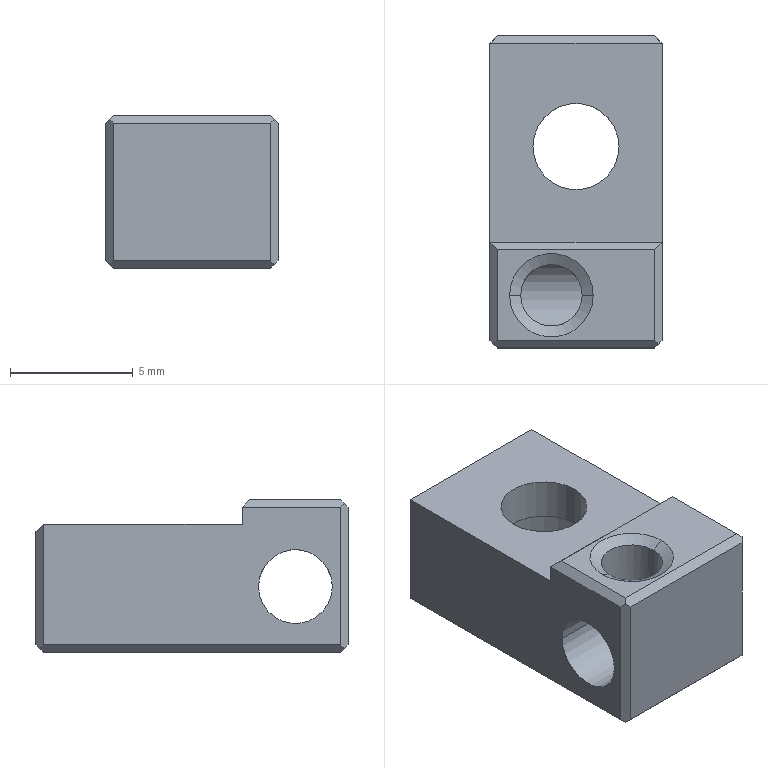Part | NX | 1 solid | 32 faces | box 7 x 12.687 x 6.2 mm | volume 311.946 mm3 | plane 22 | cylinder 8 | cone 2 | commonest cylinder face diameters 2.5 x2 3 x2 3.5 x2 6 x2
STEP:
#1=CARTESIAN_POINT('',(-50.91,-43.177,5.403));
#2=VERTEX_POINT('',#1);
#3=CARTESIAN_POINT('',(-54.31,-43.177,5.403));
#4=VERTEX_POINT('',#3);
#5=CARTESIAN_POINT('',(-52.61,-43.177,5.403));
#6=DIRECTION('',(0.,0.,1.));
#7=DIRECTION('',(1.,0.,0.));
#8=AXIS2_PLACEMENT_3D('',#5,#6,#7);
#9=CIRCLE('',#8,1.7);
#10=EDGE_CURVE('',#2,#4,#9,.T.);
#11=ORIENTED_EDGE('',*,*,#10,.T.);
#12=CARTESIAN_POINT('',(-53.86,-43.177,5.143));
#13=VERTEX_POINT('',#12);
#14=CARTESIAN_POINT('',(-53.86,-43.177,5.143));
#15=DIRECTION('',(-0.866,0.,0.5));
#16=VECTOR('',#15,1000.);
#17=LINE('',#14,#16);
#18=EDGE_CURVE('',#4,#13,#17,.F.);
#19=ORIENTED_EDGE('',*,*,#18,.T.);
#20=CARTESIAN_POINT('',(-51.36,-43.177,5.143));
#21=VERTEX_POINT('',#20);
#22=CARTESIAN_POINT('',(-52.61,-43.177,5.143));
#23=DIRECTION('',(0.,0.,1.));
#24=DIRECTION('',(1.,0.,0.));
#25=AXIS2_PLACEMENT_3D('',#22,#23,#24);
#26=CIRCLE('',#25,1.25);
#27=EDGE_CURVE('',#21,#13,#26,.T.);
#28=ORIENTED_EDGE('',*,*,#27,.F.);
#29=CARTESIAN_POINT('',(-51.36,-43.177,5.143));
#30=DIRECTION('',(0.866,0.,0.5));
#31=VECTOR('',#30,1000.);
#32=LINE('',#29,#31);
#33=EDGE_CURVE('',#2,#21,#32,.F.);
#34=ORIENTED_EDGE('',*,*,#33,.F.);
#35=EDGE_LOOP('',(#11,#19,#28,#34));
#36=FACE_BOUND('',#35,.T.);
#37=CARTESIAN_POINT('',(-52.61,-43.177,5.143));
#38=DIRECTION('',(0.,0.,1.));
#39=DIRECTION('',(1.,0.,0.));
#40=AXIS2_PLACEMENT_3D('',#37,#38,#39);
#41=CONICAL_SURFACE('',#40,1.25,1.047);
#42=ADVANCED_FACE('',(#36),#41,.F.);
#43=CARTESIAN_POINT('',(-55.11,-32.929,-0.4969));
#44=VERTEX_POINT('',#43);
#45=CARTESIAN_POINT('',(-55.11,-32.929,4.403));
#46=VERTEX_POINT('',#45);
#47=CARTESIAN_POINT('',(-55.11,-32.929,1.803));
#48=DIRECTION('',(0.,0.,1.));
#49=VECTOR('',#48,1000.);
#50=LINE('',#47,#49);
#51=EDGE_CURVE('',#44,#46,#50,.T.);
#52=ORIENTED_EDGE('',*,*,#51,.F.);
#53=CARTESIAN_POINT('',(-55.11,-45.016,-0.4969));
#54=VERTEX_POINT('',#53);
#55=CARTESIAN_POINT('',(-55.11,-38.972,-0.4969));
#56=DIRECTION('',(0.,1.,0.));
#57=VECTOR('',#56,1000.);
#58=LINE('',#55,#57);
#59=EDGE_CURVE('',#54,#44,#58,.T.);
#60=ORIENTED_EDGE('',*,*,#59,.F.);
#61=CARTESIAN_POINT('',(-55.11,-45.016,5.103));
#62=VERTEX_POINT('',#61);
#63=CARTESIAN_POINT('',(-55.11,-45.016,2.303));
#64=DIRECTION('',(0.,0.,-1.));
#65=VECTOR('',#64,1000.);
#66=LINE('',#63,#65);
#67=EDGE_CURVE('',#62,#54,#66,.T.);
#68=ORIENTED_EDGE('',*,*,#67,.F.);
#69=CARTESIAN_POINT('',(-55.11,-41.016,5.103));
#70=VERTEX_POINT('',#69);
#71=CARTESIAN_POINT('',(-55.11,-43.166,5.103));
#72=DIRECTION('',(0.,-1.,0.));
#73=VECTOR('',#72,1000.);
#74=LINE('',#71,#73);
#75=EDGE_CURVE('',#70,#62,#74,.T.);
#76=ORIENTED_EDGE('',*,*,#75,.F.);
#77=CARTESIAN_POINT('',(-55.11,-41.016,4.403));
#78=VERTEX_POINT('',#77);
#79=CARTESIAN_POINT('',(-55.11,-41.016,3.403));
#80=DIRECTION('',(0.,0.,1.));
#81=VECTOR('',#80,1000.);
#82=LINE('',#79,#81);
#83=EDGE_CURVE('',#78,#70,#82,.T.);
#84=ORIENTED_EDGE('',*,*,#83,.F.);
#85=CARTESIAN_POINT('',(-55.11,-36.078,4.403));
#86=DIRECTION('',(0.,1.,0.));
#87=VECTOR('',#86,1000.);
#88=LINE('',#85,#87);
#89=EDGE_CURVE('',#78,#46,#88,.T.);
#90=ORIENTED_EDGE('',*,*,#89,.T.);
#91=EDGE_LOOP('',(#52,#60,#68,#76,#84,#90));
#92=FACE_BOUND('',#91,.T.);
#93=CARTESIAN_POINT('',(-55.11,-41.677,1.873));
#94=VERTEX_POINT('',#93);
#95=CARTESIAN_POINT('',(-55.11,-44.677,1.873));
#96=VERTEX_POINT('',#95);
#97=CARTESIAN_POINT('',(-55.11,-43.177,1.873));
#98=DIRECTION('',(-1.,0.,0.));
#99=DIRECTION('',(0.,-1.,0.));
#100=AXIS2_PLACEMENT_3D('',#97,#98,#99);
#101=CIRCLE('',#100,1.5);
#102=EDGE_CURVE('',#94,#96,#101,.T.);
#103=ORIENTED_EDGE('',*,*,#102,.F.);
#104=CARTESIAN_POINT('',(-55.11,-43.177,1.873));
#105=DIRECTION('',(-1.,0.,0.));
#106=DIRECTION('',(0.,-1.,0.));
#107=AXIS2_PLACEMENT_3D('',#104,#105,#106);
#108=CIRCLE('',#107,1.5);
#109=EDGE_CURVE('',#96,#94,#108,.T.);
#110=ORIENTED_EDGE('',*,*,#109,.F.);
#111=EDGE_LOOP('',(#103,#110));
#112=FACE_BOUND('',#111,.T.);
#113=CARTESIAN_POINT('',(-55.11,-32.629,3.403));
#114=DIRECTION('',(-1.,0.,0.));
#115=DIRECTION('',(0.,0.,1.));
#116=AXIS2_PLACEMENT_3D('',#113,#114,#115);
#117=PLANE('',#116);
#118=ADVANCED_FACE('',(#92,#112),#117,.T.);
#119=CARTESIAN_POINT('',(-54.81,-32.629,4.103));
#120=VERTEX_POINT('',#119);
#121=CARTESIAN_POINT('',(-48.41,-32.629,4.103));
#122=VERTEX_POINT('',#121);
#123=CARTESIAN_POINT('',(-49.386,-32.629,4.103));
#124=DIRECTION('',(1.,0.,0.));
#125=VECTOR('',#124,1000.);
#126=LINE('',#123,#125);
#127=EDGE_CURVE('',#120,#122,#126,.T.);
#128=ORIENTED_EDGE('',*,*,#127,.T.);
#129=CARTESIAN_POINT('',(-48.41,-32.629,-0.4969));
#130=VERTEX_POINT('',#129);
#131=CARTESIAN_POINT('',(-48.41,-32.629,3.403));
#132=DIRECTION('',(0.,0.,1.));
#133=VECTOR('',#132,1000.);
#134=LINE('',#131,#133);
#135=EDGE_CURVE('',#130,#122,#134,.T.);
#136=ORIENTED_EDGE('',*,*,#135,.F.);
#137=CARTESIAN_POINT('',(-54.81,-32.629,-0.4969));
#138=VERTEX_POINT('',#137);
#139=CARTESIAN_POINT('',(-49.386,-32.629,-0.4969));
#140=DIRECTION('',(-1.,0.,0.));
#141=VECTOR('',#140,1000.);
#142=LINE('',#139,#141);
#143=EDGE_CURVE('',#130,#138,#142,.T.);
#144=ORIENTED_EDGE('',*,*,#143,.T.);
#145=CARTESIAN_POINT('',(-54.81,-32.629,1.803));
#146=DIRECTION('',(0.,0.,1.));
#147=VECTOR('',#146,1000.);
#148=LINE('',#145,#147);
#149=EDGE_CURVE('',#138,#120,#148,.T.);
#150=ORIENTED_EDGE('',*,*,#149,.T.);
#151=EDGE_LOOP('',(#128,#136,#144,#150));
#152=FACE_BOUND('',#151,.T.);
#153=CARTESIAN_POINT('',(-48.11,-32.629,3.403));
#154=DIRECTION('',(0.,1.,0.));
#155=DIRECTION('',(0.,0.,-1.));
#156=AXIS2_PLACEMENT_3D('',#153,#154,#155);
#157=PLANE('',#156);
#158=ADVANCED_FACE('',(#152),#157,.T.);
#159=CARTESIAN_POINT('',(-48.11,-32.929,-0.4969));
#160=VERTEX_POINT('',#159);
#161=CARTESIAN_POINT('',(-48.11,-32.929,4.403));
#162=VERTEX_POINT('',#161);
#163=CARTESIAN_POINT('',(-48.11,-32.929,3.403));
#164=DIRECTION('',(0.,0.,1.));
#165=VECTOR('',#164,1000.);
#166=LINE('',#163,#165);
#167=EDGE_CURVE('',#160,#162,#166,.T.);
#168=ORIENTED_EDGE('',*,*,#167,.T.);
#169=CARTESIAN_POINT('',(-48.11,-41.016,4.403));
#170=VERTEX_POINT('',#169);
#171=CARTESIAN_POINT('',(-48.11,-36.078,4.403));
#172=DIRECTION('',(0.,1.,0.));
#173=VECTOR('',#172,1000.);
#174=LINE('',#171,#173);
#175=EDGE_CURVE('',#170,#162,#174,.T.);
#176=ORIENTED_EDGE('',*,*,#175,.F.);
#177=CARTESIAN_POINT('',(-48.11,-41.016,5.103));
#178=VERTEX_POINT('',#177);
#179=CARTESIAN_POINT('',(-48.11,-41.016,3.403));
#180=DIRECTION('',(0.,0.,-1.));
#181=VECTOR('',#180,1000.);
#182=LINE('',#179,#181);
#183=EDGE_CURVE('',#178,#170,#182,.T.);
#184=ORIENTED_EDGE('',*,*,#183,.F.);
#185=CARTESIAN_POINT('',(-48.11,-45.016,5.103));
#186=VERTEX_POINT('',#185);
#187=CARTESIAN_POINT('',(-48.11,-43.166,5.103));
#188=DIRECTION('',(0.,-1.,0.));
#189=VECTOR('',#188,1000.);
#190=LINE('',#187,#189);
#191=EDGE_CURVE('',#178,#186,#190,.T.);
#192=ORIENTED_EDGE('',*,*,#191,.T.);
#193=CARTESIAN_POINT('',(-48.11,-45.016,-0.4969));
#194=VERTEX_POINT('',#193);
#195=CARTESIAN_POINT('',(-48.11,-45.016,3.403));
#196=DIRECTION('',(0.,0.,-1.));
#197=VECTOR('',#196,1000.);
#198=LINE('',#195,#197);
#199=EDGE_CURVE('',#186,#194,#198,.T.);
#200=ORIENTED_EDGE('',*,*,#199,.T.);
#201=CARTESIAN_POINT('',(-48.11,-38.972,-0.4969));
#202=DIRECTION('',(0.,1.,0.));
#203=VECTOR('',#202,1000.);
#204=LINE('',#201,#203);
#205=EDGE_CURVE('',#194,#160,#204,.T.);
#206=ORIENTED_EDGE('',*,*,#205,.T.);
#207=EDGE_LOOP('',(#168,#176,#184,#192,#200,#206));
#208=FACE_BOUND('',#207,.T.);
#209=CARTESIAN_POINT('',(-48.11,-41.677,1.873));
#210=VERTEX_POINT('',#209);
#211=CARTESIAN_POINT('',(-48.11,-44.677,1.873));
#212=VERTEX_POINT('',#211);
#213=CARTESIAN_POINT('',(-48.11,-43.177,1.873));
#214=DIRECTION('',(-1.,0.,0.));
#215=DIRECTION('',(0.,-1.,0.));
#216=AXIS2_PLACEMENT_3D('',#213,#214,#215);
#217=CIRCLE('',#216,1.5);
#218=EDGE_CURVE('',#210,#212,#217,.T.);
#219=ORIENTED_EDGE('',*,*,#218,.T.);
#220=CARTESIAN_POINT('',(-48.11,-43.177,1.873));
#221=DIRECTION('',(-1.,0.,0.));
#222=DIRECTION('',(0.,-1.,0.));
#223=AXIS2_PLACEMENT_3D('',#220,#221,#222);
#224=CIRCLE('',#223,1.5);
#225=EDGE_CURVE('',#212,#210,#224,.T.);
#226=ORIENTED_EDGE('',*,*,#225,.T.);
#227=EDGE_LOOP('',(#219,#226));
#228=FACE_BOUND('',#227,.T.);
#229=CARTESIAN_POINT('',(-48.11,-52.629,3.403));
#230=DIRECTION('',(1.,0.,0.));
#231=DIRECTION('',(0.,0.,1.));
#232=AXIS2_PLACEMENT_3D('',#229,#230,#231);
#233=PLANE('',#232);
#234=ADVANCED_FACE('',(#208,#228),#233,.T.);
#235=ORIENTED_EDGE('',*,*,#218,.F.);
#236=CARTESIAN_POINT('',(-47.41,-41.677,1.873));
#237=DIRECTION('',(-1.,0.,0.));
#238=VECTOR('',#237,1000.);
#239=LINE('',#236,#238);
#240=EDGE_CURVE('',#94,#210,#239,.F.);
#241=ORIENTED_EDGE('',*,*,#240,.F.);
#242=ORIENTED_EDGE('',*,*,#102,.T.);
#243=CARTESIAN_POINT('',(-47.41,-44.677,1.873));
#244=DIRECTION('',(-1.,0.,0.));
#245=VECTOR('',#244,1000.);
#246=LINE('',#243,#245);
#247=EDGE_CURVE('',#96,#212,#246,.F.);
#248=ORIENTED_EDGE('',*,*,#247,.T.);
#249=EDGE_LOOP('',(#235,#241,#242,#248));
#250=FACE_BOUND('',#249,.T.);
#251=CARTESIAN_POINT('',(-47.41,-43.177,1.873));
#252=DIRECTION('',(-1.,0.,0.));
#253=DIRECTION('',(0.,-1.,0.));
#254=AXIS2_PLACEMENT_3D('',#251,#252,#253);
#255=CYLINDRICAL_SURFACE('',#254,1.5);
#256=ADVANCED_FACE('',(#250),#255,.F.);
#257=ORIENTED_EDGE('',*,*,#167,.F.);
#258=CARTESIAN_POINT('',(-48.26,-32.779,-0.6469));
#259=VERTEX_POINT('',#258);
#260=CARTESIAN_POINT('',(-49.386,-31.653,-1.773));
#261=DIRECTION('',(0.5774,-0.5774,0.5774));
#262=VECTOR('',#261,1000.);
#263=LINE('',#260,#262);
#264=EDGE_CURVE('',#259,#160,#263,.T.);
#265=ORIENTED_EDGE('',*,*,#264,.F.);
#266=CARTESIAN_POINT('',(-49.386,-31.653,0.4788));
#267=DIRECTION('',(0.5774,-0.5774,-0.5774));
#268=VECTOR('',#267,1000.);
#269=LINE('',#266,#268);
#270=EDGE_CURVE('',#130,#259,#269,.T.);
#271=ORIENTED_EDGE('',*,*,#270,.F.);
#272=ORIENTED_EDGE('',*,*,#135,.T.);
#273=CARTESIAN_POINT('',(-49.386,-31.653,3.127));
#274=DIRECTION('',(0.5774,-0.5774,0.5774));
#275=VECTOR('',#274,1000.);
#276=LINE('',#273,#275);
#277=EDGE_CURVE('',#122,#162,#276,.T.);
#278=ORIENTED_EDGE('',*,*,#277,.T.);
#279=EDGE_LOOP('',(#257,#265,#271,#272,#278));
#280=FACE_BOUND('',#279,.T.);
#281=CARTESIAN_POINT('',(-48.26,-32.779,1.153));
#282=DIRECTION('',(-0.7071,-0.7071,0.));
#283=DIRECTION('',(-0.7071,0.7071,0.));
#284=AXIS2_PLACEMENT_3D('',#281,#282,#283);
#285=PLANE('',#284);
#286=ADVANCED_FACE('',(#280),#285,.F.);
#287=CARTESIAN_POINT('',(-53.86,-43.177,3.373));
#288=VERTEX_POINT('',#287);
#289=CARTESIAN_POINT('',(-52.61,-44.427,2.702));
#290=VERTEX_POINT('',#289);
#291=CARTESIAN_POINT('',(-53.86,-43.177,3.373));
#292=CARTESIAN_POINT('',(-53.86,-43.199,3.373));
#293=CARTESIAN_POINT('',(-53.86,-43.22,3.373));
#294=CARTESIAN_POINT('',(-53.859,-43.242,3.372));
#295=CARTESIAN_POINT('',(-53.857,-43.264,3.371));
#296=CARTESIAN_POINT('',(-53.856,-43.286,3.369));
#297=CARTESIAN_POINT('',(-53.853,-43.307,3.367));
#298=CARTESIAN_POINT('',(-53.851,-43.329,3.365));
#299=CARTESIAN_POINT('',(-53.848,-43.35,3.363));
#300=CARTESIAN_POINT('',(-53.845,-43.372,3.36));
#301=CARTESIAN_POINT('',(-53.842,-43.393,3.358));
#302=CARTESIAN_POINT('',(-53.838,-43.414,3.354));
#303=CARTESIAN_POINT('',(-53.833,-43.435,3.351));
#304=CARTESIAN_POINT('',(-53.829,-43.457,3.347));
#305=CARTESIAN_POINT('',(-53.824,-43.478,3.343));
#306=CARTESIAN_POINT('',(-53.818,-43.498,3.338));
#307=CARTESIAN_POINT('',(-53.813,-43.519,3.334));
#308=CARTESIAN_POINT('',(-53.807,-43.539,3.329));
#309=CARTESIAN_POINT('',(-53.8,-43.56,3.323));
#310=CARTESIAN_POINT('',(-53.794,-43.58,3.318));
#311=CARTESIAN_POINT('',(-53.787,-43.6,3.312));
#312=CARTESIAN_POINT('',(-53.779,-43.619,3.306));
#313=CARTESIAN_POINT('',(-53.772,-43.639,3.3));
#314=CARTESIAN_POINT('',(-53.764,-43.658,3.294));
#315=CARTESIAN_POINT('',(-53.756,-43.677,3.287));
#316=CARTESIAN_POINT('',(-53.747,-43.696,3.28));
#317=CARTESIAN_POINT('',(-53.739,-43.715,3.273));
#318=CARTESIAN_POINT('',(-53.73,-43.733,3.266));
#319=CARTESIAN_POINT('',(-53.72,-43.752,3.259));
#320=CARTESIAN_POINT('',(-53.711,-43.77,3.251));
#321=CARTESIAN_POINT('',(-53.701,-43.788,3.243));
#322=CARTESIAN_POINT('',(-53.691,-43.805,3.235));
#323=CARTESIAN_POINT('',(-53.68,-43.823,3.227));
#324=CARTESIAN_POINT('',(-53.67,-43.84,3.218));
#325=CARTESIAN_POINT('',(-53.659,-43.857,3.21));
#326=CARTESIAN_POINT('',(-53.648,-43.874,3.201));
#327=CARTESIAN_POINT('',(-53.636,-43.89,3.192));
#328=CARTESIAN_POINT('',(-53.625,-43.907,3.183));
#329=CARTESIAN_POINT('',(-53.613,-43.923,3.174));
#330=CARTESIAN_POINT('',(-53.601,-43.939,3.165));
#331=CARTESIAN_POINT('',(-53.589,-43.954,3.156));
#332=CARTESIAN_POINT('',(-53.577,-43.97,3.146));
#333=CARTESIAN_POINT('',(-53.564,-43.985,3.137));
#334=CARTESIAN_POINT('',(-53.539,-44.014,3.118));
#335=CARTESIAN_POINT('',(-53.512,-44.043,3.098));
#336=CARTESIAN_POINT('',(-53.485,-44.07,3.078));
#337=CARTESIAN_POINT('',(-53.457,-44.097,3.058));
#338=CARTESIAN_POINT('',(-53.428,-44.123,3.037));
#339=CARTESIAN_POINT('',(-53.398,-44.147,3.017));
#340=CARTESIAN_POINT('',(-53.383,-44.16,3.006));
#341=CARTESIAN_POINT('',(-53.367,-44.171,2.996));
#342=CARTESIAN_POINT('',(-53.352,-44.183,2.986));
#343=CARTESIAN_POINT('',(-53.336,-44.194,2.975));
#344=CARTESIAN_POINT('',(-53.32,-44.205,2.965));
#345=CARTESIAN_POINT('',(-53.304,-44.216,2.954));
#346=CARTESIAN_POINT('',(-53.288,-44.227,2.944));
#347=CARTESIAN_POINT('',(-53.272,-44.237,2.934));
#348=CARTESIAN_POINT('',(-53.255,-44.247,2.924));
#349=CARTESIAN_POINT('',(-53.239,-44.257,2.913));
#350=CARTESIAN_POINT('',(-53.222,-44.267,2.903));
#351=CARTESIAN_POINT('',(-53.205,-44.276,2.893));
#352=CARTESIAN_POINT('',(-53.188,-44.285,2.884));
#353=CARTESIAN_POINT('',(-53.171,-44.294,2.874));
#354=CARTESIAN_POINT('',(-53.153,-44.303,2.864));
#355=CARTESIAN_POINT('',(-53.135,-44.311,2.854));
#356=CARTESIAN_POINT('',(-53.117,-44.319,2.845));
#357=CARTESIAN_POINT('',(-53.099,-44.327,2.836));
#358=CARTESIAN_POINT('',(-53.081,-44.335,2.826));
#359=CARTESIAN_POINT('',(-53.063,-44.342,2.817));
#360=CARTESIAN_POINT('',(-53.044,-44.349,2.809));
#361=CARTESIAN_POINT('',(-53.025,-44.356,2.8));
#362=CARTESIAN_POINT('',(-53.006,-44.363,2.792));
#363=CARTESIAN_POINT('',(-52.986,-44.369,2.784));
#364=CARTESIAN_POINT('',(-52.948,-44.381,2.768));
#365=CARTESIAN_POINT('',(-52.908,-44.391,2.753));
#366=CARTESIAN_POINT('',(-52.867,-44.4,2.741));
#367=CARTESIAN_POINT('',(-52.846,-44.404,2.735));
#368=CARTESIAN_POINT('',(-52.826,-44.408,2.729));
#369=CARTESIAN_POINT('',(-52.804,-44.411,2.725));
#370=CARTESIAN_POINT('',(-52.783,-44.415,2.72));
#371=CARTESIAN_POINT('',(-52.762,-44.418,2.716));
#372=CARTESIAN_POINT('',(-52.74,-44.42,2.712));
#373=CARTESIAN_POINT('',(-52.73,-44.421,2.711));
#374=CARTESIAN_POINT('',(-52.719,-44.422,2.709));
#375=CARTESIAN_POINT('',(-52.708,-44.423,2.708));
#376=CARTESIAN_POINT('',(-52.697,-44.424,2.707));
#377=CARTESIAN_POINT('',(-52.686,-44.424,2.706));
#378=CARTESIAN_POINT('',(-52.675,-44.425,2.705));
#379=CARTESIAN_POINT('',(-52.665,-44.426,2.704));
#380=CARTESIAN_POINT('',(-52.654,-44.426,2.703));
#381=CARTESIAN_POINT('',(-52.643,-44.426,2.703));
#382=CARTESIAN_POINT('',(-52.632,-44.426,2.702));
#383=CARTESIAN_POINT('',(-52.621,-44.427,2.702));
#384=CARTESIAN_POINT('',(-52.61,-44.427,2.702));
#385=B_SPLINE_CURVE_WITH_KNOTS('',3,(#291,#292,#293,#294,#295,#296,#297,#298,#299,#300,#301,#302,#303,#304,#305,#306,#307,#308,#309,#310,#311,#312,#313,#314,#315,#316,#317,#318,#319,#320,#321,#322,#323,#324,#325,#326,#327,#328,#329,#330,#331,#332,#333,#334,#335,#336,#337,#338,#339,#340,#341,#342,#343,#344,#345,#346,#347,#348,#349,#350,#351,#352,#353,#354,#355,#356,#357,#358,#359,#360,#361,#362,#363,#364,#365,#366,#367,#368,#369,#370,#371,#372,#373,#374,#375,#376,#377,#378,#379,#380,#381,#382,#383,#384),.UNSPECIFIED.,.F.,.F.,(4,3,3,3,3,3,3,3,3,3,3,3,3,3,3,3,3,3,3,3,3,3,3,3,3,3,3,3,3,3,3,4),(0.,0.06564,0.131,0.1964,0.262,0.3277,0.3934,0.4588,0.5241,0.5897,0.6553,0.7211,0.7868,0.8525,0.9179,1.049,1.18,1.246,1.312,1.378,1.443,1.508,1.574,1.639,1.705,1.836,1.901,1.967,2.,2.033,2.065,2.098),.UNSPECIFIED.);
#386=EDGE_CURVE('',#288,#290,#385,.T.);
#387=ORIENTED_EDGE('',*,*,#386,.F.);
#388=CARTESIAN_POINT('',(-53.86,-43.177,5.403));
#389=DIRECTION('',(0.,0.,1.));
#390=VECTOR('',#389,1000.);
#391=LINE('',#388,#390);
#392=EDGE_CURVE('',#288,#13,#391,.T.);
#393=ORIENTED_EDGE('',*,*,#392,.T.);
#394=CARTESIAN_POINT('',(-52.61,-43.177,5.143));
#395=DIRECTION('',(0.,0.,1.));
#396=DIRECTION('',(1.,0.,0.));
#397=AXIS2_PLACEMENT_3D('',#394,#395,#396);
#398=CIRCLE('',#397,1.25);
#399=EDGE_CURVE('',#13,#21,#398,.T.);
#400=ORIENTED_EDGE('',*,*,#399,.T.);
#401=CARTESIAN_POINT('',(-51.36,-43.177,3.373));
#402=VERTEX_POINT('',#401);
#403=CARTESIAN_POINT('',(-51.36,-43.177,5.403));
#404=DIRECTION('',(0.,0.,1.));
#405=VECTOR('',#404,1000.);
#406=LINE('',#403,#405);
#407=EDGE_CURVE('',#402,#21,#406,.T.);
#408=ORIENTED_EDGE('',*,*,#407,.F.);
#409=CARTESIAN_POINT('',(-52.61,-44.427,2.702));
#410=CARTESIAN_POINT('',(-52.599,-44.427,2.702));
#411=CARTESIAN_POINT('',(-52.588,-44.426,2.702));
#412=CARTESIAN_POINT('',(-52.578,-44.426,2.703));
#413=CARTESIAN_POINT('',(-52.567,-44.426,2.703));
#414=CARTESIAN_POINT('',(-52.556,-44.425,2.704));
#415=CARTESIAN_POINT('',(-52.545,-44.425,2.705));
#416=CARTESIAN_POINT('',(-52.534,-44.424,2.706));
#417=CARTESIAN_POINT('',(-52.523,-44.424,2.707));
#418=CARTESIAN_POINT('',(-52.512,-44.423,2.708));
#419=CARTESIAN_POINT('',(-52.501,-44.422,2.709));
#420=CARTESIAN_POINT('',(-52.491,-44.421,2.711));
#421=CARTESIAN_POINT('',(-52.48,-44.42,2.712));
#422=CARTESIAN_POINT('',(-52.458,-44.418,2.716));
#423=CARTESIAN_POINT('',(-52.437,-44.415,2.72));
#424=CARTESIAN_POINT('',(-52.416,-44.411,2.725));
#425=CARTESIAN_POINT('',(-52.395,-44.408,2.73));
#426=CARTESIAN_POINT('',(-52.374,-44.404,2.735));
#427=CARTESIAN_POINT('',(-52.354,-44.4,2.741));
#428=CARTESIAN_POINT('',(-52.313,-44.391,2.753));
#429=CARTESIAN_POINT('',(-52.273,-44.381,2.768));
#430=CARTESIAN_POINT('',(-52.234,-44.369,2.784));
#431=CARTESIAN_POINT('',(-52.215,-44.363,2.792));
#432=CARTESIAN_POINT('',(-52.196,-44.356,2.8));
#433=CARTESIAN_POINT('',(-52.177,-44.349,2.809));
#434=CARTESIAN_POINT('',(-52.158,-44.342,2.817));
#435=CARTESIAN_POINT('',(-52.139,-44.335,2.826));
#436=CARTESIAN_POINT('',(-52.121,-44.327,2.836));
#437=CARTESIAN_POINT('',(-52.103,-44.319,2.845));
#438=CARTESIAN_POINT('',(-52.085,-44.311,2.854));
#439=CARTESIAN_POINT('',(-52.067,-44.303,2.864));
#440=CARTESIAN_POINT('',(-52.05,-44.294,2.874));
#441=CARTESIAN_POINT('',(-52.033,-44.285,2.884));
#442=CARTESIAN_POINT('',(-52.016,-44.276,2.893));
#443=CARTESIAN_POINT('',(-51.998,-44.267,2.903));
#444=CARTESIAN_POINT('',(-51.982,-44.257,2.913));
#445=CARTESIAN_POINT('',(-51.965,-44.247,2.924));
#446=CARTESIAN_POINT('',(-51.949,-44.237,2.934));
#447=CARTESIAN_POINT('',(-51.932,-44.227,2.944));
#448=CARTESIAN_POINT('',(-51.916,-44.216,2.954));
#449=CARTESIAN_POINT('',(-51.9,-44.205,2.965));
#450=CARTESIAN_POINT('',(-51.884,-44.194,2.975));
#451=CARTESIAN_POINT('',(-51.869,-44.183,2.985));
#452=CARTESIAN_POINT('',(-51.853,-44.171,2.996));
#453=CARTESIAN_POINT('',(-51.838,-44.16,3.006));
#454=CARTESIAN_POINT('',(-51.823,-44.147,3.017));
#455=CARTESIAN_POINT('',(-51.793,-44.123,3.037));
#456=CARTESIAN_POINT('',(-51.764,-44.097,3.058));
#457=CARTESIAN_POINT('',(-51.736,-44.07,3.078));
#458=CARTESIAN_POINT('',(-51.708,-44.043,3.098));
#459=CARTESIAN_POINT('',(-51.682,-44.014,3.118));
#460=CARTESIAN_POINT('',(-51.656,-43.985,3.137));
#461=CARTESIAN_POINT('',(-51.644,-43.97,3.146));
#462=CARTESIAN_POINT('',(-51.631,-43.954,3.156));
#463=CARTESIAN_POINT('',(-51.619,-43.939,3.165));
#464=CARTESIAN_POINT('',(-51.607,-43.923,3.174));
#465=CARTESIAN_POINT('',(-51.596,-43.907,3.183));
#466=CARTESIAN_POINT('',(-51.584,-43.891,3.192));
#467=CARTESIAN_POINT('',(-51.573,-43.874,3.201));
#468=CARTESIAN_POINT('',(-51.562,-43.857,3.21));
#469=CARTESIAN_POINT('',(-51.551,-43.84,3.218));
#470=CARTESIAN_POINT('',(-51.54,-43.823,3.227));
#471=CARTESIAN_POINT('',(-51.53,-43.806,3.235));
#472=CARTESIAN_POINT('',(-51.52,-43.788,3.243));
#473=CARTESIAN_POINT('',(-51.51,-43.77,3.251));
#474=CARTESIAN_POINT('',(-51.5,-43.752,3.259));
#475=CARTESIAN_POINT('',(-51.491,-43.733,3.266));
#476=CARTESIAN_POINT('',(-51.482,-43.715,3.273));
#477=CARTESIAN_POINT('',(-51.473,-43.696,3.28));
#478=CARTESIAN_POINT('',(-51.465,-43.677,3.287));
#479=CARTESIAN_POINT('',(-51.448,-43.639,3.301));
#480=CARTESIAN_POINT('',(-51.433,-43.6,3.313));
#481=CARTESIAN_POINT('',(-51.42,-43.56,3.323));
#482=CARTESIAN_POINT('',(-51.414,-43.539,3.329));
#483=CARTESIAN_POINT('',(-51.408,-43.519,3.334));
#484=CARTESIAN_POINT('',(-51.402,-43.498,3.338));
#485=CARTESIAN_POINT('',(-51.397,-43.478,3.343));
#486=CARTESIAN_POINT('',(-51.392,-43.457,3.347));
#487=CARTESIAN_POINT('',(-51.387,-43.436,3.351));
#488=CARTESIAN_POINT('',(-51.383,-43.414,3.354));
#489=CARTESIAN_POINT('',(-51.379,-43.393,3.358));
#490=CARTESIAN_POINT('',(-51.376,-43.372,3.36));
#491=CARTESIAN_POINT('',(-51.372,-43.35,3.363));
#492=CARTESIAN_POINT('',(-51.369,-43.329,3.366));
#493=CARTESIAN_POINT('',(-51.367,-43.307,3.367));
#494=CARTESIAN_POINT('',(-51.365,-43.285,3.369));
#495=CARTESIAN_POINT('',(-51.363,-43.264,3.371));
#496=CARTESIAN_POINT('',(-51.362,-43.242,3.372));
#497=CARTESIAN_POINT('',(-51.361,-43.22,3.373));
#498=CARTESIAN_POINT('',(-51.36,-43.198,3.373));
#499=CARTESIAN_POINT('',(-51.36,-43.177,3.373));
#500=B_SPLINE_CURVE_WITH_KNOTS('',3,(#409,#410,#411,#412,#413,#414,#415,#416,#417,#418,#419,#420,#421,#422,#423,#424,#425,#426,#427,#428,#429,#430,#431,#432,#433,#434,#435,#436,#437,#438,#439,#440,#441,#442,#443,#444,#445,#446,#447,#448,#449,#450,#451,#452,#453,#454,#455,#456,#457,#458,#459,#460,#461,#462,#463,#464,#465,#466,#467,#468,#469,#470,#471,#472,#473,#474,#475,#476,#477,#478,#479,#480,#481,#482,#483,#484,#485,#486,#487,#488,#489,#490,#491,#492,#493,#494,#495,#496,#497,#498,#499),.UNSPECIFIED.,.F.,.F.,(4,3,3,3,3,3,3,3,3,3,3,3,3,3,3,3,3,3,3,3,3,3,3,3,3,3,3,3,3,3,4),(0.,0.03265,0.06539,0.0982,0.1311,0.1968,0.2623,0.393,0.4586,0.5242,0.5897,0.655,0.7204,0.786,0.8518,0.9176,1.049,1.18,1.245,1.311,1.377,1.442,1.508,1.574,1.705,1.77,1.836,1.902,1.967,2.033,2.098),.UNSPECIFIED.);
#501=EDGE_CURVE('',#290,#402,#500,.T.);
#502=ORIENTED_EDGE('',*,*,#501,.F.);
#503=EDGE_LOOP('',(#387,#393,#400,#408,#502));
#504=FACE_BOUND('',#503,.T.);
#505=CARTESIAN_POINT('',(-52.61,-43.177,5.403));
#506=DIRECTION('',(0.,0.,1.));
#507=DIRECTION('',(1.,0.,0.));
#508=AXIS2_PLACEMENT_3D('',#505,#506,#507);
#509=CYLINDRICAL_SURFACE('',#508,1.25);
#510=ADVANCED_FACE('',(#504),#509,.F.);
#511=ORIENTED_EDGE('',*,*,#51,.T.);
#512=CARTESIAN_POINT('',(-49.386,-27.205,-1.321));
#513=DIRECTION('',(0.5774,0.5774,-0.5774));
#514=VECTOR('',#513,1000.);
#515=LINE('',#512,#514);
#516=EDGE_CURVE('',#46,#120,#515,.T.);
#517=ORIENTED_EDGE('',*,*,#516,.T.);
#518=ORIENTED_EDGE('',*,*,#149,.F.);
#519=CARTESIAN_POINT('',(-54.96,-32.779,-0.6469));
#520=VERTEX_POINT('',#519);
#521=CARTESIAN_POINT('',(-49.386,-27.205,4.927));
#522=DIRECTION('',(-0.5774,-0.5774,-0.5774));
#523=VECTOR('',#522,1000.);
#524=LINE('',#521,#523);
#525=EDGE_CURVE('',#138,#520,#524,.T.);
#526=ORIENTED_EDGE('',*,*,#525,.T.);
#527=CARTESIAN_POINT('',(-49.386,-27.205,-6.221));
#528=DIRECTION('',(0.5774,0.5774,-0.5774));
#529=VECTOR('',#528,1000.);
#530=LINE('',#527,#529);
#531=EDGE_CURVE('',#44,#520,#530,.T.);
#532=ORIENTED_EDGE('',*,*,#531,.F.);
#533=EDGE_LOOP('',(#511,#517,#518,#526,#532));
#534=FACE_BOUND('',#533,.T.);
#535=CARTESIAN_POINT('',(-54.96,-32.779,1.803));
#536=DIRECTION('',(0.7071,-0.7071,0.));
#537=DIRECTION('',(0.,0.,-1.));
#538=AXIS2_PLACEMENT_3D('',#535,#536,#537);
#539=PLANE('',#538);
#540=ADVANCED_FACE('',(#534),#539,.F.);
#541=ORIENTED_EDGE('',*,*,#516,.F.);
#542=CARTESIAN_POINT('',(-49.386,-32.929,4.403));
#543=DIRECTION('',(1.,0.,0.));
#544=VECTOR('',#543,1000.);
#545=LINE('',#542,#544);
#546=EDGE_CURVE('',#46,#162,#545,.T.);
#547=ORIENTED_EDGE('',*,*,#546,.T.);
#548=ORIENTED_EDGE('',*,*,#277,.F.);
#549=ORIENTED_EDGE('',*,*,#127,.F.);
#550=EDGE_LOOP('',(#541,#547,#548,#549));
#551=FACE_BOUND('',#550,.T.);
#552=CARTESIAN_POINT('',(-51.61,-32.779,4.253));
#553=DIRECTION('',(0.,-0.7071,-0.7071));
#554=DIRECTION('',(0.,0.7071,-0.7071));
#555=AXIS2_PLACEMENT_3D('',#552,#553,#554);
#556=PLANE('',#555);
#557=ADVANCED_FACE('',(#551),#556,.F.);
#558=CARTESIAN_POINT('',(-48.61,-37.129,2.703));
#559=VERTEX_POINT('',#558);
#560=CARTESIAN_POINT('',(-54.61,-37.129,2.703));
#561=VERTEX_POINT('',#560);
#562=CARTESIAN_POINT('',(-51.61,-37.129,2.703));
#563=DIRECTION('',(0.,0.,-1.));
#564=DIRECTION('',(-1.,0.,0.));
#565=AXIS2_PLACEMENT_3D('',#562,#563,#564);
#566=CIRCLE('',#565,3.);
#567=EDGE_CURVE('',#559,#561,#566,.T.);
#568=ORIENTED_EDGE('',*,*,#567,.T.);
#569=CARTESIAN_POINT('',(-51.61,-37.129,2.703));
#570=DIRECTION('',(0.,0.,-1.));
#571=DIRECTION('',(-1.,0.,0.));
#572=AXIS2_PLACEMENT_3D('',#569,#570,#571);
#573=CIRCLE('',#572,3.);
#574=EDGE_CURVE('',#561,#559,#573,.T.);
#575=ORIENTED_EDGE('',*,*,#574,.T.);
#576=EDGE_LOOP('',(#568,#575));
#577=FACE_BOUND('',#576,.T.);
#578=CARTESIAN_POINT('',(-49.86,-37.129,2.703));
#579=VERTEX_POINT('',#578);
#580=CARTESIAN_POINT('',(-53.36,-37.129,2.703));
#581=VERTEX_POINT('',#580);
#582=CARTESIAN_POINT('',(-51.61,-37.129,2.703));
#583=DIRECTION('',(0.,0.,-1.));
#584=DIRECTION('',(-1.,0.,0.));
#585=AXIS2_PLACEMENT_3D('',#582,#583,#584);
#586=CIRCLE('',#585,1.75);
#587=EDGE_CURVE('',#579,#581,#586,.T.);
#588=ORIENTED_EDGE('',*,*,#587,.F.);
#589=CARTESIAN_POINT('',(-51.61,-37.129,2.703));
#590=DIRECTION('',(0.,0.,-1.));
#591=DIRECTION('',(-1.,0.,0.));
#592=AXIS2_PLACEMENT_3D('',#589,#590,#591);
#593=CIRCLE('',#592,1.75);
#594=EDGE_CURVE('',#581,#579,#593,.T.);
#595=ORIENTED_EDGE('',*,*,#594,.F.);
#596=EDGE_LOOP('',(#588,#595));
#597=FACE_BOUND('',#596,.T.);
#598=CARTESIAN_POINT('',(-51.61,-37.129,2.703));
#599=DIRECTION('',(0.,0.,-1.));
#600=DIRECTION('',(0.,-1.,0.));
#601=AXIS2_PLACEMENT_3D('',#598,#599,#600);
#602=PLANE('',#601);
#603=ADVANCED_FACE('',(#577,#597),#602,.T.);
#604=ORIENTED_EDGE('',*,*,#587,.T.);
#605=CARTESIAN_POINT('',(-53.36,-37.129,4.403));
#606=VERTEX_POINT('',#605);
#607=CARTESIAN_POINT('',(-53.36,-37.129,-1.597));
#608=DIRECTION('',(0.,0.,-1.));
#609=VECTOR('',#608,1000.);
#610=LINE('',#607,#609);
#611=EDGE_CURVE('',#581,#606,#610,.F.);
#612=ORIENTED_EDGE('',*,*,#611,.T.);
#613=CARTESIAN_POINT('',(-49.86,-37.129,4.403));
#614=VERTEX_POINT('',#613);
#615=CARTESIAN_POINT('',(-51.61,-37.129,4.403));
#616=DIRECTION('',(0.,0.,-1.));
#617=DIRECTION('',(-1.,0.,0.));
#618=AXIS2_PLACEMENT_3D('',#615,#616,#617);
#619=CIRCLE('',#618,1.75);
#620=EDGE_CURVE('',#614,#606,#619,.T.);
#621=ORIENTED_EDGE('',*,*,#620,.F.);
#622=CARTESIAN_POINT('',(-49.86,-37.129,-1.597));
#623=DIRECTION('',(0.,0.,-1.));
#624=VECTOR('',#623,1000.);
#625=LINE('',#622,#624);
#626=EDGE_CURVE('',#579,#614,#625,.F.);
#627=ORIENTED_EDGE('',*,*,#626,.F.);
#628=EDGE_LOOP('',(#604,#612,#621,#627));
#629=FACE_BOUND('',#628,.T.);
#630=CARTESIAN_POINT('',(-51.61,-37.129,-1.597));
#631=DIRECTION('',(0.,0.,-1.));
#632=DIRECTION('',(-1.,0.,0.));
#633=AXIS2_PLACEMENT_3D('',#630,#631,#632);
#634=CYLINDRICAL_SURFACE('',#633,1.75);
#635=ADVANCED_FACE('',(#629),#634,.F.);
#636=CARTESIAN_POINT('',(-54.81,-45.016,-0.7969));
#637=VERTEX_POINT('',#636);
#638=CARTESIAN_POINT('',(-54.81,-32.929,-0.7969));
#639=VERTEX_POINT('',#638);
#640=CARTESIAN_POINT('',(-54.81,-38.972,-0.7969));
#641=DIRECTION('',(0.,1.,0.));
#642=VECTOR('',#641,1000.);
#643=LINE('',#640,#642);
#644=EDGE_CURVE('',#637,#639,#643,.T.);
#645=ORIENTED_EDGE('',*,*,#644,.T.);
#646=CARTESIAN_POINT('',(-48.41,-32.929,-0.7969));
#647=VERTEX_POINT('',#646);
#648=CARTESIAN_POINT('',(-49.386,-32.929,-0.7969));
#649=DIRECTION('',(-1.,0.,0.));
#650=VECTOR('',#649,1000.);
#651=LINE('',#648,#650);
#652=EDGE_CURVE('',#647,#639,#651,.T.);
#653=ORIENTED_EDGE('',*,*,#652,.F.);
#654=CARTESIAN_POINT('',(-48.41,-45.016,-0.7969));
#655=VERTEX_POINT('',#654);
#656=CARTESIAN_POINT('',(-48.41,-38.972,-0.7969));
#657=DIRECTION('',(0.,1.,0.));
#658=VECTOR('',#657,1000.);
#659=LINE('',#656,#658);
#660=EDGE_CURVE('',#655,#647,#659,.T.);
#661=ORIENTED_EDGE('',*,*,#660,.F.);
#662=CARTESIAN_POINT('',(-49.386,-45.016,-0.7969));
#663=DIRECTION('',(1.,0.,0.));
#664=VECTOR('',#663,1000.);
#665=LINE('',#662,#664);
#666=EDGE_CURVE('',#637,#655,#665,.T.);
#667=ORIENTED_EDGE('',*,*,#666,.F.);
#668=EDGE_LOOP('',(#645,#653,#661,#667));
#669=FACE_BOUND('',#668,.T.);
#670=CARTESIAN_POINT('',(-54.61,-37.129,-0.7969));
#671=VERTEX_POINT('',#670);
#672=CARTESIAN_POINT('',(-48.61,-37.129,-0.7969));
#673=VERTEX_POINT('',#672);
#674=CARTESIAN_POINT('',(-51.61,-37.129,-0.7969));
#675=DIRECTION('',(0.,0.,-1.));
#676=DIRECTION('',(-1.,0.,0.));
#677=AXIS2_PLACEMENT_3D('',#674,#675,#676);
#678=CIRCLE('',#677,3.);
#679=EDGE_CURVE('',#671,#673,#678,.T.);
#680=ORIENTED_EDGE('',*,*,#679,.F.);
#681=CARTESIAN_POINT('',(-51.61,-37.129,-0.7969));
#682=DIRECTION('',(0.,0.,-1.));
#683=DIRECTION('',(-1.,0.,0.));
#684=AXIS2_PLACEMENT_3D('',#681,#682,#683);
#685=CIRCLE('',#684,3.);
#686=EDGE_CURVE('',#673,#671,#685,.T.);
#687=ORIENTED_EDGE('',*,*,#686,.F.);
#688=EDGE_LOOP('',(#680,#687));
#689=FACE_BOUND('',#688,.T.);
#690=CARTESIAN_POINT('',(-49.386,-36.078,-0.7969));
#691=DIRECTION('',(0.,0.,-1.));
#692=DIRECTION('',(0.,-1.,0.));
#693=AXIS2_PLACEMENT_3D('',#690,#691,#692);
#694=PLANE('',#693);
#695=ADVANCED_FACE('',(#669,#689),#694,.T.);
#696=CARTESIAN_POINT('',(-54.81,-45.316,5.103));
#697=VERTEX_POINT('',#696);
#698=CARTESIAN_POINT('',(-54.81,-45.316,-0.4969));
#699=VERTEX_POINT('',#698);
#700=CARTESIAN_POINT('',(-54.81,-45.316,2.303));
#701=DIRECTION('',(0.,0.,-1.));
#702=VECTOR('',#701,1000.);
#703=LINE('',#700,#702);
#704=EDGE_CURVE('',#697,#699,#703,.T.);
#705=ORIENTED_EDGE('',*,*,#704,.T.);
#706=CARTESIAN_POINT('',(-48.41,-45.316,-0.4969));
#707=VERTEX_POINT('',#706);
#708=CARTESIAN_POINT('',(-49.386,-45.316,-0.4969));
#709=DIRECTION('',(1.,0.,0.));
#710=VECTOR('',#709,1000.);
#711=LINE('',#708,#710);
#712=EDGE_CURVE('',#699,#707,#711,.T.);
#713=ORIENTED_EDGE('',*,*,#712,.T.);
#714=CARTESIAN_POINT('',(-48.41,-45.316,5.103));
#715=VERTEX_POINT('',#714);
#716=CARTESIAN_POINT('',(-48.41,-45.316,3.403));
#717=DIRECTION('',(0.,0.,-1.));
#718=VECTOR('',#717,1000.);
#719=LINE('',#716,#718);
#720=EDGE_CURVE('',#715,#707,#719,.T.);
#721=ORIENTED_EDGE('',*,*,#720,.F.);
#722=CARTESIAN_POINT('',(-49.386,-45.316,5.103));
#723=DIRECTION('',(-1.,0.,0.));
#724=VECTOR('',#723,1000.);
#725=LINE('',#722,#724);
#726=EDGE_CURVE('',#715,#697,#725,.T.);
#727=ORIENTED_EDGE('',*,*,#726,.T.);
#728=EDGE_LOOP('',(#705,#713,#721,#727));
#729=FACE_BOUND('',#728,.T.);
#730=CARTESIAN_POINT('',(-33.55,-45.316,3.403));
#731=DIRECTION('',(0.,-1.,0.));
#732=DIRECTION('',(-1.,0.,0.));
#733=AXIS2_PLACEMENT_3D('',#730,#731,#732);
#734=PLANE('',#733);
#735=ADVANCED_FACE('',(#729),#734,.T.);
#736=CARTESIAN_POINT('',(-54.81,-41.316,5.403));
#737=VERTEX_POINT('',#736);
#738=CARTESIAN_POINT('',(-54.81,-45.016,5.403));
#739=VERTEX_POINT('',#738);
#740=CARTESIAN_POINT('',(-54.81,-43.166,5.403));
#741=DIRECTION('',(0.,-1.,0.));
#742=VECTOR('',#741,1000.);
#743=LINE('',#740,#742);
#744=EDGE_CURVE('',#737,#739,#743,.T.);
#745=ORIENTED_EDGE('',*,*,#744,.T.);
#746=CARTESIAN_POINT('',(-48.41,-45.016,5.403));
#747=VERTEX_POINT('',#746);
#748=CARTESIAN_POINT('',(-49.386,-45.016,5.403));
#749=DIRECTION('',(-1.,0.,0.));
#750=VECTOR('',#749,1000.);
#751=LINE('',#748,#750);
#752=EDGE_CURVE('',#747,#739,#751,.T.);
#753=ORIENTED_EDGE('',*,*,#752,.F.);
#754=CARTESIAN_POINT('',(-48.41,-41.316,5.403));
#755=VERTEX_POINT('',#754);
#756=CARTESIAN_POINT('',(-48.41,-43.166,5.403));
#757=DIRECTION('',(0.,-1.,0.));
#758=VECTOR('',#757,1000.);
#759=LINE('',#756,#758);
#760=EDGE_CURVE('',#755,#747,#759,.T.);
#761=ORIENTED_EDGE('',*,*,#760,.F.);
#762=CARTESIAN_POINT('',(-49.386,-41.316,5.403));
#763=DIRECTION('',(1.,0.,0.));
#764=VECTOR('',#763,1000.);
#765=LINE('',#762,#764);
#766=EDGE_CURVE('',#737,#755,#765,.T.);
#767=ORIENTED_EDGE('',*,*,#766,.F.);
#768=EDGE_LOOP('',(#745,#753,#761,#767));
#769=FACE_BOUND('',#768,.T.);
#770=ORIENTED_EDGE('',*,*,#10,.F.);
#771=CARTESIAN_POINT('',(-52.61,-43.177,5.403));
#772=DIRECTION('',(0.,0.,1.));
#773=DIRECTION('',(1.,0.,0.));
#774=AXIS2_PLACEMENT_3D('',#771,#772,#773);
#775=CIRCLE('',#774,1.7);
#776=EDGE_CURVE('',#4,#2,#775,.T.);
#777=ORIENTED_EDGE('',*,*,#776,.F.);
#778=EDGE_LOOP('',(#770,#777));
#779=FACE_BOUND('',#778,.T.);
#780=CARTESIAN_POINT('',(-52.759,-43.092,5.403));
#781=DIRECTION('',(0.,0.,1.));
#782=DIRECTION('',(1.,0.,0.));
#783=AXIS2_PLACEMENT_3D('',#780,#781,#782);
#784=PLANE('',#783);
#785=ADVANCED_FACE('',(#769,#779),#784,.T.);
#786=ORIENTED_EDGE('',*,*,#652,.T.);
#787=CARTESIAN_POINT('',(-51.661,-36.078,-3.946));
#788=DIRECTION('',(-0.5774,0.5774,0.5774));
#789=VECTOR('',#788,1000.);
#790=LINE('',#787,#789);
#791=EDGE_CURVE('',#639,#520,#790,.T.);
#792=ORIENTED_EDGE('',*,*,#791,.T.);
#793=ORIENTED_EDGE('',*,*,#525,.F.);
#794=ORIENTED_EDGE('',*,*,#143,.F.);
#795=ORIENTED_EDGE('',*,*,#270,.T.);
#796=CARTESIAN_POINT('',(-49.386,-33.905,-1.773));
#797=DIRECTION('',(0.5774,0.5774,0.5774));
#798=VECTOR('',#797,1000.);
#799=LINE('',#796,#798);
#800=EDGE_CURVE('',#647,#259,#799,.T.);
#801=ORIENTED_EDGE('',*,*,#800,.F.);
#802=EDGE_LOOP('',(#786,#792,#793,#794,#795,#801));
#803=FACE_BOUND('',#802,.T.);
#804=CARTESIAN_POINT('',(-52.61,-32.779,-0.6469));
#805=DIRECTION('',(0.,-0.7071,0.7071));
#806=DIRECTION('',(-1.,0.,0.));
#807=AXIS2_PLACEMENT_3D('',#804,#805,#806);
#808=PLANE('',#807);
#809=ADVANCED_FACE('',(#803),#808,.F.);
#810=CARTESIAN_POINT('',(-49.386,-41.016,5.103));
#811=DIRECTION('',(1.,0.,0.));
#812=VECTOR('',#811,1000.);
#813=LINE('',#810,#812);
#814=EDGE_CURVE('',#70,#178,#813,.T.);
#815=ORIENTED_EDGE('',*,*,#814,.F.);
#816=CARTESIAN_POINT('',(-56.81,-39.316,3.403));
#817=DIRECTION('',(0.5774,-0.5774,0.5774));
#818=VECTOR('',#817,1000.);
#819=LINE('',#816,#818);
#820=EDGE_CURVE('',#70,#737,#819,.T.);
#821=ORIENTED_EDGE('',*,*,#820,.T.);
#822=ORIENTED_EDGE('',*,*,#766,.T.);
#823=CARTESIAN_POINT('',(-46.41,-39.316,3.403));
#824=DIRECTION('',(-0.5774,-0.5774,0.5774));
#825=VECTOR('',#824,1000.);
#826=LINE('',#823,#825);
#827=EDGE_CURVE('',#178,#755,#826,.T.);
#828=ORIENTED_EDGE('',*,*,#827,.F.);
#829=EDGE_LOOP('',(#815,#821,#822,#828));
#830=FACE_BOUND('',#829,.T.);
#831=CARTESIAN_POINT('',(-51.61,-41.166,5.253));
#832=DIRECTION('',(0.,-0.7071,-0.7071));
#833=DIRECTION('',(0.,0.7071,-0.7071));
#834=AXIS2_PLACEMENT_3D('',#831,#832,#833);
#835=PLANE('',#834);
#836=ADVANCED_FACE('',(#830),#835,.F.);
#837=ORIENTED_EDGE('',*,*,#660,.T.);
#838=ORIENTED_EDGE('',*,*,#800,.T.);
#839=ORIENTED_EDGE('',*,*,#264,.T.);
#840=ORIENTED_EDGE('',*,*,#205,.F.);
#841=CARTESIAN_POINT('',(-48.26,-45.166,-0.6469));
#842=VERTEX_POINT('',#841);
#843=CARTESIAN_POINT('',(-49.386,-46.292,-1.773));
#844=DIRECTION('',(-0.5774,-0.5774,-0.5774));
#845=VECTOR('',#844,1000.);
#846=LINE('',#843,#845);
#847=EDGE_CURVE('',#194,#842,#846,.T.);
#848=ORIENTED_EDGE('',*,*,#847,.T.);
#849=CARTESIAN_POINT('',(-57.348,-36.078,-9.735));
#850=DIRECTION('',(-0.5774,0.5774,-0.5774));
#851=VECTOR('',#850,1000.);
#852=LINE('',#849,#851);
#853=EDGE_CURVE('',#842,#655,#852,.T.);
#854=ORIENTED_EDGE('',*,*,#853,.T.);
#855=EDGE_LOOP('',(#837,#838,#839,#840,#848,#854));
#856=FACE_BOUND('',#855,.T.);
#857=CARTESIAN_POINT('',(-48.26,-38.972,-0.6469));
#858=DIRECTION('',(-0.7071,0.,0.7071));
#859=DIRECTION('',(0.,1.,0.));
#860=AXIS2_PLACEMENT_3D('',#857,#858,#859);
#861=PLANE('',#860);
#862=ADVANCED_FACE('',(#856),#861,.F.);
#863=ORIENTED_EDGE('',*,*,#760,.T.);
#864=CARTESIAN_POINT('',(-48.26,-45.166,5.253));
#865=VERTEX_POINT('',#864);
#866=CARTESIAN_POINT('',(-57.348,-36.078,14.341));
#867=DIRECTION('',(-0.5774,0.5774,0.5774));
#868=VECTOR('',#867,1000.);
#869=LINE('',#866,#868);
#870=EDGE_CURVE('',#865,#747,#869,.T.);
#871=ORIENTED_EDGE('',*,*,#870,.F.);
#872=CARTESIAN_POINT('',(-46.41,-43.316,3.403));
#873=DIRECTION('',(-0.5774,-0.5774,0.5774));
#874=VECTOR('',#873,1000.);
#875=LINE('',#872,#874);
#876=EDGE_CURVE('',#186,#865,#875,.T.);
#877=ORIENTED_EDGE('',*,*,#876,.F.);
#878=ORIENTED_EDGE('',*,*,#191,.F.);
#879=ORIENTED_EDGE('',*,*,#827,.T.);
#880=EDGE_LOOP('',(#863,#871,#877,#878,#879));
#881=FACE_BOUND('',#880,.T.);
#882=CARTESIAN_POINT('',(-48.26,-43.166,5.253));
#883=DIRECTION('',(-0.7071,0.,-0.7071));
#884=DIRECTION('',(-0.7071,0.,0.7071));
#885=AXIS2_PLACEMENT_3D('',#882,#883,#884);
#886=PLANE('',#885);
#887=ADVANCED_FACE('',(#881),#886,.F.);
#888=ORIENTED_EDGE('',*,*,#752,.T.);
#889=CARTESIAN_POINT('',(-54.96,-45.166,5.253));
#890=VERTEX_POINT('',#889);
#891=CARTESIAN_POINT('',(-49.386,-39.592,10.827));
#892=DIRECTION('',(-0.5774,-0.5774,-0.5774));
#893=VECTOR('',#892,1000.);
#894=LINE('',#891,#893);
#895=EDGE_CURVE('',#739,#890,#894,.T.);
#896=ORIENTED_EDGE('',*,*,#895,.T.);
#897=CARTESIAN_POINT('',(-64.048,-36.078,14.341));
#898=DIRECTION('',(0.5774,-0.5774,-0.5774));
#899=VECTOR('',#898,1000.);
#900=LINE('',#897,#899);
#901=EDGE_CURVE('',#890,#697,#900,.T.);
#902=ORIENTED_EDGE('',*,*,#901,.T.);
#903=ORIENTED_EDGE('',*,*,#726,.F.);
#904=CARTESIAN_POINT('',(-49.386,-46.292,4.127));
#905=DIRECTION('',(-0.5774,-0.5774,-0.5774));
#906=VECTOR('',#905,1000.);
#907=LINE('',#904,#906);
#908=EDGE_CURVE('',#865,#715,#907,.T.);
#909=ORIENTED_EDGE('',*,*,#908,.F.);
#910=ORIENTED_EDGE('',*,*,#870,.T.);
#911=EDGE_LOOP('',(#888,#896,#902,#903,#909,#910));
#912=FACE_BOUND('',#911,.T.);
#913=CARTESIAN_POINT('',(-51.61,-45.166,5.253));
#914=DIRECTION('',(0.,0.7071,-0.7071));
#915=DIRECTION('',(-1.,0.,0.));
#916=AXIS2_PLACEMENT_3D('',#913,#914,#915);
#917=PLANE('',#916);
#918=ADVANCED_FACE('',(#912),#917,.F.);
#919=ORIENTED_EDGE('',*,*,#720,.T.);
#920=CARTESIAN_POINT('',(-49.386,-46.292,0.4788));
#921=DIRECTION('',(-0.5774,-0.5774,0.5774));
#922=VECTOR('',#921,1000.);
#923=LINE('',#920,#922);
#924=EDGE_CURVE('',#842,#707,#923,.T.);
#925=ORIENTED_EDGE('',*,*,#924,.F.);
#926=ORIENTED_EDGE('',*,*,#847,.F.);
#927=ORIENTED_EDGE('',*,*,#199,.F.);
#928=ORIENTED_EDGE('',*,*,#876,.T.);
#929=ORIENTED_EDGE('',*,*,#908,.T.);
#930=EDGE_LOOP('',(#919,#925,#926,#927,#928,#929));
#931=FACE_BOUND('',#930,.T.);
#932=CARTESIAN_POINT('',(-48.26,-45.166,1.653));
#933=DIRECTION('',(-0.7071,0.7071,0.));
#934=DIRECTION('',(0.,0.,1.));
#935=AXIS2_PLACEMENT_3D('',#932,#933,#934);
#936=PLANE('',#935);
#937=ADVANCED_FACE('',(#931),#936,.F.);
#938=ORIENTED_EDGE('',*,*,#712,.F.);
#939=CARTESIAN_POINT('',(-54.96,-45.166,-0.6469));
#940=VERTEX_POINT('',#939);
#941=CARTESIAN_POINT('',(-64.048,-36.078,-9.735));
#942=DIRECTION('',(-0.5774,0.5774,-0.5774));
#943=VECTOR('',#942,1000.);
#944=LINE('',#941,#943);
#945=EDGE_CURVE('',#699,#940,#944,.T.);
#946=ORIENTED_EDGE('',*,*,#945,.T.);
#947=CARTESIAN_POINT('',(-49.386,-39.592,-6.221));
#948=DIRECTION('',(0.5774,0.5774,-0.5774));
#949=VECTOR('',#948,1000.);
#950=LINE('',#947,#949);
#951=EDGE_CURVE('',#940,#637,#950,.T.);
#952=ORIENTED_EDGE('',*,*,#951,.T.);
#953=ORIENTED_EDGE('',*,*,#666,.T.);
#954=ORIENTED_EDGE('',*,*,#853,.F.);
#955=ORIENTED_EDGE('',*,*,#924,.T.);
#956=EDGE_LOOP('',(#938,#946,#952,#953,#954,#955));
#957=FACE_BOUND('',#956,.T.);
#958=CARTESIAN_POINT('',(-52.61,-45.166,-0.6469));
#959=DIRECTION('',(0.,0.7071,0.7071));
#960=DIRECTION('',(1.,0.,0.));
#961=AXIS2_PLACEMENT_3D('',#958,#959,#960);
#962=PLANE('',#961);
#963=ADVANCED_FACE('',(#957),#962,.F.);
#964=ORIENTED_EDGE('',*,*,#644,.F.);
#965=ORIENTED_EDGE('',*,*,#951,.F.);
#966=CARTESIAN_POINT('',(-64.048,-36.078,8.441));
#967=DIRECTION('',(0.5774,-0.5774,-0.5774));
#968=VECTOR('',#967,1000.);
#969=LINE('',#966,#968);
#970=EDGE_CURVE('',#54,#940,#969,.T.);
#971=ORIENTED_EDGE('',*,*,#970,.F.);
#972=ORIENTED_EDGE('',*,*,#59,.T.);
#973=ORIENTED_EDGE('',*,*,#531,.T.);
#974=ORIENTED_EDGE('',*,*,#791,.F.);
#975=EDGE_LOOP('',(#964,#965,#971,#972,#973,#974));
#976=FACE_BOUND('',#975,.T.);
#977=CARTESIAN_POINT('',(-54.96,-38.972,-0.6469));
#978=DIRECTION('',(-0.7071,0.,-0.7071));
#979=DIRECTION('',(-0.7071,0.,0.7071));
#980=AXIS2_PLACEMENT_3D('',#977,#978,#979);
#981=PLANE('',#980);
#982=ADVANCED_FACE('',(#976),#981,.T.);
#983=ORIENTED_EDGE('',*,*,#704,.F.);
#984=ORIENTED_EDGE('',*,*,#901,.F.);
#985=CARTESIAN_POINT('',(-64.048,-36.078,-3.835));
#986=DIRECTION('',(0.5774,-0.5774,0.5774));
#987=VECTOR('',#986,1000.);
#988=LINE('',#985,#987);
#989=EDGE_CURVE('',#62,#890,#988,.T.);
#990=ORIENTED_EDGE('',*,*,#989,.F.);
#991=ORIENTED_EDGE('',*,*,#67,.T.);
#992=ORIENTED_EDGE('',*,*,#970,.T.);
#993=ORIENTED_EDGE('',*,*,#945,.F.);
#994=EDGE_LOOP('',(#983,#984,#990,#991,#992,#993));
#995=FACE_BOUND('',#994,.T.);
#996=CARTESIAN_POINT('',(-54.96,-45.166,2.303));
#997=DIRECTION('',(-0.7071,-0.7071,0.));
#998=DIRECTION('',(-0.7071,0.7071,0.));
#999=AXIS2_PLACEMENT_3D('',#996,#997,#998);
#1000=PLANE('',#999);
#1001=ADVANCED_FACE('',(#995),#1000,.T.);
#1002=ORIENTED_EDGE('',*,*,#744,.F.);
#1003=ORIENTED_EDGE('',*,*,#820,.F.);
#1004=ORIENTED_EDGE('',*,*,#75,.T.);
#1005=ORIENTED_EDGE('',*,*,#989,.T.);
#1006=ORIENTED_EDGE('',*,*,#895,.F.);
#1007=EDGE_LOOP('',(#1002,#1003,#1004,#1005,#1006));
#1008=FACE_BOUND('',#1007,.T.);
#1009=CARTESIAN_POINT('',(-54.96,-43.166,5.253));
#1010=DIRECTION('',(-0.7071,0.,0.7071));
#1011=DIRECTION('',(0.,1.,0.));
#1012=AXIS2_PLACEMENT_3D('',#1009,#1010,#1011);
#1013=PLANE('',#1012);
#1014=ADVANCED_FACE('',(#1008),#1013,.T.);
#1015=ORIENTED_EDGE('',*,*,#679,.T.);
#1016=CARTESIAN_POINT('',(-48.61,-37.129,-1.597));
#1017=DIRECTION('',(0.,0.,-1.));
#1018=VECTOR('',#1017,1000.);
#1019=LINE('',#1016,#1018);
#1020=EDGE_CURVE('',#559,#673,#1019,.T.);
#1021=ORIENTED_EDGE('',*,*,#1020,.F.);
#1022=ORIENTED_EDGE('',*,*,#574,.F.);
#1023=CARTESIAN_POINT('',(-54.61,-37.129,-1.597));
#1024=DIRECTION('',(0.,0.,-1.));
#1025=VECTOR('',#1024,1000.);
#1026=LINE('',#1023,#1025);
#1027=EDGE_CURVE('',#561,#671,#1026,.T.);
#1028=ORIENTED_EDGE('',*,*,#1027,.T.);
#1029=EDGE_LOOP('',(#1015,#1021,#1022,#1028));
#1030=FACE_BOUND('',#1029,.T.);
#1031=CARTESIAN_POINT('',(-51.61,-37.129,-1.597));
#1032=DIRECTION('',(0.,0.,-1.));
#1033=DIRECTION('',(-1.,0.,0.));
#1034=AXIS2_PLACEMENT_3D('',#1031,#1032,#1033);
#1035=CYLINDRICAL_SURFACE('',#1034,3.);
#1036=ADVANCED_FACE('',(#1030),#1035,.F.);
#1037=ORIENTED_EDGE('',*,*,#546,.F.);
#1038=ORIENTED_EDGE('',*,*,#89,.F.);
#1039=CARTESIAN_POINT('',(-49.386,-41.016,4.403));
#1040=DIRECTION('',(-1.,0.,0.));
#1041=VECTOR('',#1040,1000.);
#1042=LINE('',#1039,#1041);
#1043=EDGE_CURVE('',#170,#78,#1042,.T.);
#1044=ORIENTED_EDGE('',*,*,#1043,.F.);
#1045=ORIENTED_EDGE('',*,*,#175,.T.);
#1046=EDGE_LOOP('',(#1037,#1038,#1044,#1045));
#1047=FACE_BOUND('',#1046,.T.);
#1048=CARTESIAN_POINT('',(-51.61,-37.129,4.403));
#1049=DIRECTION('',(0.,0.,-1.));
#1050=DIRECTION('',(-1.,0.,0.));
#1051=AXIS2_PLACEMENT_3D('',#1048,#1049,#1050);
#1052=CIRCLE('',#1051,1.75);
#1053=EDGE_CURVE('',#606,#614,#1052,.T.);
#1054=ORIENTED_EDGE('',*,*,#1053,.T.);
#1055=ORIENTED_EDGE('',*,*,#620,.T.);
#1056=EDGE_LOOP('',(#1054,#1055));
#1057=FACE_BOUND('',#1056,.T.);
#1058=CARTESIAN_POINT('',(-49.386,-36.078,4.403));
#1059=DIRECTION('',(0.,0.,-1.));
#1060=DIRECTION('',(0.,-1.,0.));
#1061=AXIS2_PLACEMENT_3D('',#1058,#1059,#1060);
#1062=PLANE('',#1061);
#1063=ADVANCED_FACE('',(#1047,#1057),#1062,.F.);
#1064=ORIENTED_EDGE('',*,*,#1043,.T.);
#1065=ORIENTED_EDGE('',*,*,#83,.T.);
#1066=ORIENTED_EDGE('',*,*,#814,.T.);
#1067=ORIENTED_EDGE('',*,*,#183,.T.);
#1068=EDGE_LOOP('',(#1064,#1065,#1066,#1067));
#1069=FACE_BOUND('',#1068,.T.);
#1070=CARTESIAN_POINT('',(-54.11,-41.016,3.403));
#1071=DIRECTION('',(0.,1.,0.));
#1072=DIRECTION('',(1.,0.,0.));
#1073=AXIS2_PLACEMENT_3D('',#1070,#1071,#1072);
#1074=PLANE('',#1073);
#1075=ADVANCED_FACE('',(#1069),#1074,.T.);
#1076=ORIENTED_EDGE('',*,*,#567,.F.);
#1077=ORIENTED_EDGE('',*,*,#1020,.T.);
#1078=ORIENTED_EDGE('',*,*,#686,.T.);
#1079=ORIENTED_EDGE('',*,*,#1027,.F.);
#1080=EDGE_LOOP('',(#1076,#1077,#1078,#1079));
#1081=FACE_BOUND('',#1080,.T.);
#1082=CARTESIAN_POINT('',(-51.61,-37.129,-1.597));
#1083=DIRECTION('',(0.,0.,-1.));
#1084=DIRECTION('',(-1.,0.,0.));
#1085=AXIS2_PLACEMENT_3D('',#1082,#1083,#1084);
#1086=CYLINDRICAL_SURFACE('',#1085,3.);
#1087=ADVANCED_FACE('',(#1081),#1086,.F.);
#1088=ORIENTED_EDGE('',*,*,#247,.F.);
#1089=ORIENTED_EDGE('',*,*,#109,.T.);
#1090=ORIENTED_EDGE('',*,*,#240,.T.);
#1091=ORIENTED_EDGE('',*,*,#225,.F.);
#1092=EDGE_LOOP('',(#1088,#1089,#1090,#1091));
#1093=FACE_BOUND('',#1092,.T.);
#1094=ORIENTED_EDGE('',*,*,#386,.T.);
#1095=ORIENTED_EDGE('',*,*,#501,.T.);
#1096=CARTESIAN_POINT('',(-51.36,-43.177,3.373));
#1097=CARTESIAN_POINT('',(-51.36,-43.148,3.373));
#1098=CARTESIAN_POINT('',(-51.361,-43.12,3.372));
#1099=CARTESIAN_POINT('',(-51.363,-43.092,3.371));
#1100=CARTESIAN_POINT('',(-51.364,-43.077,3.37));
#1101=CARTESIAN_POINT('',(-51.365,-43.062,3.369));
#1102=CARTESIAN_POINT('',(-51.367,-43.047,3.367));
#1103=CARTESIAN_POINT('',(-51.369,-43.032,3.366));
#1104=CARTESIAN_POINT('',(-51.37,-43.017,3.365));
#1105=CARTESIAN_POINT('',(-51.373,-43.002,3.363));
#1106=CARTESIAN_POINT('',(-51.375,-42.987,3.361));
#1107=CARTESIAN_POINT('',(-51.377,-42.972,3.359));
#1108=CARTESIAN_POINT('',(-51.38,-42.957,3.357));
#1109=CARTESIAN_POINT('',(-51.382,-42.942,3.355));
#1110=CARTESIAN_POINT('',(-51.385,-42.928,3.352));
#1111=CARTESIAN_POINT('',(-51.388,-42.913,3.35));
#1112=CARTESIAN_POINT('',(-51.395,-42.884,3.345));
#1113=CARTESIAN_POINT('',(-51.402,-42.855,3.339));
#1114=CARTESIAN_POINT('',(-51.41,-42.827,3.332));
#1115=CARTESIAN_POINT('',(-51.418,-42.798,3.325));
#1116=CARTESIAN_POINT('',(-51.428,-42.771,3.317));
#1117=CARTESIAN_POINT('',(-51.438,-42.743,3.309));
#1118=CARTESIAN_POINT('',(-51.448,-42.716,3.301));
#1119=CARTESIAN_POINT('',(-51.459,-42.689,3.292));
#1120=CARTESIAN_POINT('',(-51.471,-42.662,3.282));
#1121=CARTESIAN_POINT('',(-51.483,-42.636,3.273));
#1122=CARTESIAN_POINT('',(-51.495,-42.611,3.262));
#1123=CARTESIAN_POINT('',(-51.509,-42.586,3.252));
#1124=CARTESIAN_POINT('',(-51.516,-42.573,3.246));
#1125=CARTESIAN_POINT('',(-51.522,-42.561,3.241));
#1126=CARTESIAN_POINT('',(-51.529,-42.549,3.235));
#1127=CARTESIAN_POINT('',(-51.536,-42.537,3.23));
#1128=CARTESIAN_POINT('',(-51.544,-42.525,3.224));
#1129=CARTESIAN_POINT('',(-51.551,-42.513,3.218));
#1130=CARTESIAN_POINT('',(-51.566,-42.489,3.206));
#1131=CARTESIAN_POINT('',(-51.582,-42.466,3.194));
#1132=CARTESIAN_POINT('',(-51.598,-42.444,3.182));
#1133=CARTESIAN_POINT('',(-51.616,-42.419,3.168));
#1134=CARTESIAN_POINT('',(-51.635,-42.394,3.153));
#1135=CARTESIAN_POINT('',(-51.654,-42.371,3.138));
#1136=CARTESIAN_POINT('',(-51.674,-42.348,3.124));
#1137=CARTESIAN_POINT('',(-51.695,-42.325,3.108));
#1138=CARTESIAN_POINT('',(-51.716,-42.304,3.093));
#1139=CARTESIAN_POINT('',(-51.737,-42.282,3.077));
#1140=CARTESIAN_POINT('',(-51.758,-42.261,3.062));
#1141=CARTESIAN_POINT('',(-51.781,-42.241,3.046));
#1142=CARTESIAN_POINT('',(-51.792,-42.232,3.038));
#1143=CARTESIAN_POINT('',(-51.803,-42.222,3.03));
#1144=CARTESIAN_POINT('',(-51.815,-42.212,3.022));
#1145=CARTESIAN_POINT('',(-51.826,-42.203,3.014));
#1146=CARTESIAN_POINT('',(-51.838,-42.194,3.006));
#1147=CARTESIAN_POINT('',(-51.85,-42.185,2.998));
#1148=CARTESIAN_POINT('',(-51.873,-42.166,2.982));
#1149=CARTESIAN_POINT('',(-51.898,-42.149,2.966));
#1150=CARTESIAN_POINT('',(-51.923,-42.133,2.95));
#1151=CARTESIAN_POINT('',(-51.948,-42.116,2.934));
#1152=CARTESIAN_POINT('',(-51.973,-42.101,2.918));
#1153=CARTESIAN_POINT('',(-52.,-42.086,2.903));
#1154=CARTESIAN_POINT('',(-52.026,-42.071,2.887));
#1155=CARTESIAN_POINT('',(-52.053,-42.057,2.872));
#1156=CARTESIAN_POINT('',(-52.081,-42.044,2.857));
#1157=CARTESIAN_POINT('',(-52.108,-42.032,2.842));
#1158=CARTESIAN_POINT('',(-52.136,-42.02,2.828));
#1159=CARTESIAN_POINT('',(-52.165,-42.009,2.814));
#1160=CARTESIAN_POINT('',(-52.182,-42.002,2.806));
#1161=CARTESIAN_POINT('',(-52.199,-41.996,2.799));
#1162=CARTESIAN_POINT('',(-52.216,-41.99,2.791));
#1163=CARTESIAN_POINT('',(-52.233,-41.985,2.784));
#1164=CARTESIAN_POINT('',(-52.251,-41.979,2.777));
#1165=CARTESIAN_POINT('',(-52.269,-41.974,2.77));
#1166=CARTESIAN_POINT('',(-52.286,-41.969,2.763));
#1167=CARTESIAN_POINT('',(-52.304,-41.964,2.757));
#1168=CARTESIAN_POINT('',(-52.323,-41.96,2.751));
#1169=CARTESIAN_POINT('',(-52.341,-41.956,2.745));
#1170=CARTESIAN_POINT('',(-52.36,-41.952,2.739));
#1171=CARTESIAN_POINT('',(-52.378,-41.948,2.734));
#1172=CARTESIAN_POINT('',(-52.397,-41.945,2.729));
#1173=CARTESIAN_POINT('',(-52.416,-41.942,2.725));
#1174=CARTESIAN_POINT('',(-52.435,-41.939,2.721));
#1175=CARTESIAN_POINT('',(-52.454,-41.936,2.717));
#1176=CARTESIAN_POINT('',(-52.473,-41.934,2.713));
#1177=CARTESIAN_POINT('',(-52.492,-41.932,2.711));
#1178=CARTESIAN_POINT('',(-52.512,-41.93,2.708));
#1179=CARTESIAN_POINT('',(-52.531,-41.929,2.706));
#1180=CARTESIAN_POINT('',(-52.551,-41.928,2.704));
#1181=CARTESIAN_POINT('',(-52.57,-41.927,2.703));
#1182=CARTESIAN_POINT('',(-52.59,-41.927,2.702));
#1183=CARTESIAN_POINT('',(-52.61,-41.927,2.702));
#1184=CARTESIAN_POINT('',(-52.63,-41.927,2.702));
#1185=CARTESIAN_POINT('',(-52.649,-41.927,2.703));
#1186=CARTESIAN_POINT('',(-52.669,-41.928,2.704));
#1187=CARTESIAN_POINT('',(-52.689,-41.929,2.706));
#1188=CARTESIAN_POINT('',(-52.708,-41.93,2.708));
#1189=CARTESIAN_POINT('',(-52.728,-41.932,2.711));
#1190=CARTESIAN_POINT('',(-52.747,-41.934,2.713));
#1191=CARTESIAN_POINT('',(-52.766,-41.936,2.717));
#1192=CARTESIAN_POINT('',(-52.785,-41.939,2.72));
#1193=CARTESIAN_POINT('',(-52.804,-41.942,2.724));
#1194=CARTESIAN_POINT('',(-52.823,-41.945,2.729));
#1195=CARTESIAN_POINT('',(-52.842,-41.948,2.734));
#1196=CARTESIAN_POINT('',(-52.86,-41.952,2.739));
#1197=CARTESIAN_POINT('',(-52.879,-41.956,2.744));
#1198=CARTESIAN_POINT('',(-52.897,-41.96,2.75));
#1199=CARTESIAN_POINT('',(-52.915,-41.964,2.756));
#1200=CARTESIAN_POINT('',(-52.933,-41.969,2.763));
#1201=CARTESIAN_POINT('',(-52.951,-41.974,2.77));
#1202=CARTESIAN_POINT('',(-52.969,-41.979,2.776));
#1203=CARTESIAN_POINT('',(-52.987,-41.984,2.783));
#1204=CARTESIAN_POINT('',(-53.004,-41.99,2.791));
#1205=CARTESIAN_POINT('',(-53.021,-41.996,2.798));
#1206=CARTESIAN_POINT('',(-53.038,-42.002,2.806));
#1207=CARTESIAN_POINT('',(-53.055,-42.008,2.814));
#1208=CARTESIAN_POINT('',(-53.084,-42.019,2.827));
#1209=CARTESIAN_POINT('',(-53.112,-42.031,2.842));
#1210=CARTESIAN_POINT('',(-53.139,-42.044,2.857));
#1211=CARTESIAN_POINT('',(-53.167,-42.057,2.871));
#1212=CARTESIAN_POINT('',(-53.194,-42.071,2.887));
#1213=CARTESIAN_POINT('',(-53.22,-42.086,2.902));
#1214=CARTESIAN_POINT('',(-53.246,-42.1,2.918));
#1215=CARTESIAN_POINT('',(-53.272,-42.116,2.934));
#1216=CARTESIAN_POINT('',(-53.297,-42.132,2.95));
#1217=CARTESIAN_POINT('',(-53.322,-42.149,2.966));
#1218=CARTESIAN_POINT('',(-53.346,-42.166,2.982));
#1219=CARTESIAN_POINT('',(-53.37,-42.184,2.998));
#1220=CARTESIAN_POINT('',(-53.382,-42.193,3.006));
#1221=CARTESIAN_POINT('',(-53.394,-42.202,3.014));
#1222=CARTESIAN_POINT('',(-53.405,-42.212,3.022));
#1223=CARTESIAN_POINT('',(-53.417,-42.221,3.03));
#1224=CARTESIAN_POINT('',(-53.428,-42.231,3.038));
#1225=CARTESIAN_POINT('',(-53.439,-42.241,3.045));
#1226=CARTESIAN_POINT('',(-53.461,-42.261,3.061));
#1227=CARTESIAN_POINT('',(-53.483,-42.281,3.077));
#1228=CARTESIAN_POINT('',(-53.504,-42.303,3.092));
#1229=CARTESIAN_POINT('',(-53.525,-42.325,3.108));
#1230=CARTESIAN_POINT('',(-53.546,-42.347,3.123));
#1231=CARTESIAN_POINT('',(-53.566,-42.371,3.138));
#1232=CARTESIAN_POINT('',(-53.585,-42.394,3.153));
#1233=CARTESIAN_POINT('',(-53.604,-42.418,3.167));
#1234=CARTESIAN_POINT('',(-53.622,-42.443,3.182));
#1235=CARTESIAN_POINT('',(-53.639,-42.466,3.194));
#1236=CARTESIAN_POINT('',(-53.654,-42.489,3.206));
#1237=CARTESIAN_POINT('',(-53.669,-42.512,3.218));
#1238=CARTESIAN_POINT('',(-53.684,-42.536,3.23));
#1239=CARTESIAN_POINT('',(-53.698,-42.56,3.241));
#1240=CARTESIAN_POINT('',(-53.711,-42.585,3.252));
#1241=CARTESIAN_POINT('',(-53.725,-42.61,3.262));
#1242=CARTESIAN_POINT('',(-53.737,-42.636,3.272));
#1243=CARTESIAN_POINT('',(-53.749,-42.662,3.282));
#1244=CARTESIAN_POINT('',(-53.761,-42.688,3.292));
#1245=CARTESIAN_POINT('',(-53.772,-42.715,3.301));
#1246=CARTESIAN_POINT('',(-53.782,-42.743,3.309));
#1247=CARTESIAN_POINT('',(-53.793,-42.77,3.317));
#1248=CARTESIAN_POINT('',(-53.802,-42.798,3.325));
#1249=CARTESIAN_POINT('',(-53.81,-42.826,3.332));
#1250=CARTESIAN_POINT('',(-53.819,-42.855,3.338));
#1251=CARTESIAN_POINT('',(-53.826,-42.884,3.345));
#1252=CARTESIAN_POINT('',(-53.832,-42.913,3.35));
#1253=CARTESIAN_POINT('',(-53.835,-42.928,3.352));
#1254=CARTESIAN_POINT('',(-53.838,-42.942,3.355));
#1255=CARTESIAN_POINT('',(-53.841,-42.957,3.357));
#1256=CARTESIAN_POINT('',(-53.843,-42.972,3.359));
#1257=CARTESIAN_POINT('',(-53.846,-42.986,3.361));
#1258=CARTESIAN_POINT('',(-53.848,-43.001,3.363));
#1259=CARTESIAN_POINT('',(-53.85,-43.016,3.365));
#1260=CARTESIAN_POINT('',(-53.852,-43.031,3.366));
#1261=CARTESIAN_POINT('',(-53.853,-43.046,3.367));
#1262=CARTESIAN_POINT('',(-53.855,-43.061,3.369));
#1263=CARTESIAN_POINT('',(-53.856,-43.076,3.37));
#1264=CARTESIAN_POINT('',(-53.857,-43.091,3.371));
#1265=CARTESIAN_POINT('',(-53.859,-43.12,3.372));
#1266=CARTESIAN_POINT('',(-53.86,-43.148,3.373));
#1267=CARTESIAN_POINT('',(-53.86,-43.177,3.373));
#1268=B_SPLINE_CURVE_WITH_KNOTS('',3,(#1096,#1097,#1098,#1099,#1100,#1101,#1102,#1103,#1104,#1105,#1106,#1107,#1108,#1109,#1110,#1111,#1112,#1113,#1114,#1115,#1116,#1117,#1118,#1119,#1120,#1121,#1122,#1123,#1124,#1125,#1126,#1127,#1128,#1129,#1130,#1131,#1132,#1133,#1134,#1135,#1136,#1137,#1138,#1139,#1140,#1141,#1142,#1143,#1144,#1145,#1146,#1147,#1148,#1149,#1150,#1151,#1152,#1153,#1154,#1155,#1156,#1157,#1158,#1159,#1160,#1161,#1162,#1163,#1164,#1165,#1166,#1167,#1168,#1169,#1170,#1171,#1172,#1173,#1174,#1175,#1176,#1177,#1178,#1179,#1180,#1181,#1182,#1183,#1184,#1185,#1186,#1187,#1188,#1189,#1190,#1191,#1192,#1193,#1194,#1195,#1196,#1197,#1198,#1199,#1200,#1201,#1202,#1203,#1204,#1205,#1206,#1207,#1208,#1209,#1210,#1211,#1212,#1213,#1214,#1215,#1216,#1217,#1218,#1219,#1220,#1221,#1222,#1223,#1224,#1225,#1226,#1227,#1228,#1229,#1230,#1231,#1232,#1233,#1234,#1235,#1236,#1237,#1238,#1239,#1240,#1241,#1242,#1243,#1244,#1245,#1246,#1247,#1248,#1249,#1250,#1251,#1252,#1253,#1254,#1255,#1256,#1257,#1258,#1259,#1260,#1261,#1262,#1263,#1264,#1265,#1266,#1267),.UNSPECIFIED.,.F.,.F.,(4,3,3,3,3,3,3,3,3,3,3,3,3,3,3,3,3,3,3,3,3,3,3,3,3,3,3,3,3,3,3,3,3,3,3,3,3,3,3,3,3,3,3,3,3,3,3,3,3,3,3,3,3,3,3,3,3,4),(0.,0.08477,0.1304,0.176,0.2215,0.2669,0.3577,0.4488,0.54,0.631,0.6763,0.7217,0.8127,0.9145,1.016,1.118,1.169,1.219,1.321,1.423,1.524,1.626,1.685,1.744,1.803,1.862,1.921,1.98,2.038,2.098,2.157,2.216,2.275,2.334,2.393,2.452,2.511,2.57,2.671,2.772,2.874,2.976,3.027,3.077,3.179,3.281,3.383,3.474,3.565,3.655,3.747,3.838,3.929,3.974,4.02,4.065,4.111,4.196),.UNSPECIFIED.);
#1269=EDGE_CURVE('',#402,#288,#1268,.T.);
#1270=ORIENTED_EDGE('',*,*,#1269,.T.);
#1271=EDGE_LOOP('',(#1094,#1095,#1270));
#1272=FACE_BOUND('',#1271,.T.);
#1273=CARTESIAN_POINT('',(-47.41,-43.177,1.873));
#1274=DIRECTION('',(-1.,0.,0.));
#1275=DIRECTION('',(0.,-1.,0.));
#1276=AXIS2_PLACEMENT_3D('',#1273,#1274,#1275);
#1277=CYLINDRICAL_SURFACE('',#1276,1.5);
#1278=ADVANCED_FACE('',(#1093,#1272),#1277,.F.);
#1279=ORIENTED_EDGE('',*,*,#1053,.F.);
#1280=ORIENTED_EDGE('',*,*,#611,.F.);
#1281=ORIENTED_EDGE('',*,*,#594,.T.);
#1282=ORIENTED_EDGE('',*,*,#626,.T.);
#1283=EDGE_LOOP('',(#1279,#1280,#1281,#1282));
#1284=FACE_BOUND('',#1283,.T.);
#1285=CARTESIAN_POINT('',(-51.61,-37.129,-1.597));
#1286=DIRECTION('',(0.,0.,-1.));
#1287=DIRECTION('',(-1.,0.,0.));
#1288=AXIS2_PLACEMENT_3D('',#1285,#1286,#1287);
#1289=CYLINDRICAL_SURFACE('',#1288,1.75);
#1290=ADVANCED_FACE('',(#1284),#1289,.F.);
#1291=ORIENTED_EDGE('',*,*,#399,.F.);
#1292=ORIENTED_EDGE('',*,*,#18,.F.);
#1293=ORIENTED_EDGE('',*,*,#776,.T.);
#1294=ORIENTED_EDGE('',*,*,#33,.T.);
#1295=EDGE_LOOP('',(#1291,#1292,#1293,#1294));
#1296=FACE_BOUND('',#1295,.T.);
#1297=CARTESIAN_POINT('',(-52.61,-43.177,5.143));
#1298=DIRECTION('',(0.,0.,1.));
#1299=DIRECTION('',(1.,0.,0.));
#1300=AXIS2_PLACEMENT_3D('',#1297,#1298,#1299);
#1301=CONICAL_SURFACE('',#1300,1.25,1.047);
#1302=ADVANCED_FACE('',(#1296),#1301,.F.);
#1303=ORIENTED_EDGE('',*,*,#407,.T.);
#1304=ORIENTED_EDGE('',*,*,#27,.T.);
#1305=ORIENTED_EDGE('',*,*,#392,.F.);
#1306=ORIENTED_EDGE('',*,*,#1269,.F.);
#1307=EDGE_LOOP('',(#1303,#1304,#1305,#1306));
#1308=FACE_BOUND('',#1307,.T.);
#1309=CARTESIAN_POINT('',(-52.61,-43.177,5.403));
#1310=DIRECTION('',(0.,0.,1.));
#1311=DIRECTION('',(1.,0.,0.));
#1312=AXIS2_PLACEMENT_3D('',#1309,#1310,#1311);
#1313=CYLINDRICAL_SURFACE('',#1312,1.25);
#1314=ADVANCED_FACE('',(#1308),#1313,.F.);
#1315=CLOSED_SHELL('',(#42,#118,#158,#234,#256,#286,#510,#540,#557,#603,#635,#695,#735,#785,#809,#836,#862,#887,#918,#937,#963,#982,#1001,#1014,#1036,#1063,#1075,#1087,#1278,#1290,#1302,#1314));
#1316=MANIFOLD_SOLID_BREP('',#1315);
#1317=(LENGTH_UNIT()NAMED_UNIT(*)SI_UNIT(.MILLI.,.METRE.));
#1318=UNCERTAINTY_MEASURE_WITH_UNIT(LENGTH_MEASURE(0.00001),#1317,'','');
#1319=(NAMED_UNIT(*)PLANE_ANGLE_UNIT()SI_UNIT($,.RADIAN.));
#1320=(NAMED_UNIT(*)SI_UNIT($,.STERADIAN.)SOLID_ANGLE_UNIT());
#1321=(GEOMETRIC_REPRESENTATION_CONTEXT(3)GLOBAL_UNCERTAINTY_ASSIGNED_CONTEXT((#1318))GLOBAL_UNIT_ASSIGNED_CONTEXT((#1317,#1319,#1320))REPRESENTATION_CONTEXT('',''));
#1322=ADVANCED_BREP_SHAPE_REPRESENTATION('',(#1316),#1321);